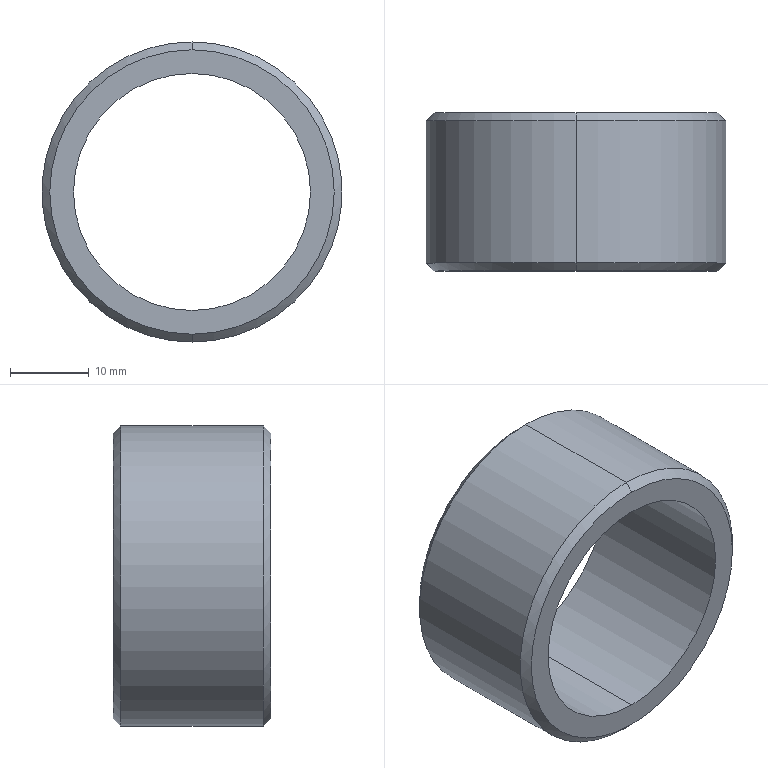Part | SolidWorks | features Chamfer 1, Extrusion 1 | 1 solid | 10 faces | box 38 x 20 x 38 mm | volume 8428 mm3 | cone 4 | cylinder 4 | plane 2 | commonest cylinder face diameters 30 x2 38 x2
STEP:
#1=CARTESIAN_POINT('',(0.,20.,18.));
#2=VERTEX_POINT('',#1);
#3=CARTESIAN_POINT('',(0.,20.,-18.));
#4=VERTEX_POINT('',#3);
#5=CARTESIAN_POINT('',(0.,20.,0.));
#6=DIRECTION('',(0.,1.,0.));
#7=DIRECTION('',(0.,0.,1.));
#8=AXIS2_PLACEMENT_3D('',#5,#6,#7);
#9=CIRCLE('',#8,18.);
#10=EDGE_CURVE('',#2,#4,#9,.T.);
#11=ORIENTED_EDGE('',*,*,#10,.F.);
#12=CARTESIAN_POINT('',(0.,19.,19.));
#13=VERTEX_POINT('',#12);
#14=CARTESIAN_POINT('',(0.,20.,18.));
#15=DIRECTION('',(0.,-0.7071,0.7071));
#16=VECTOR('',#15,1000.);
#17=LINE('',#14,#16);
#18=EDGE_CURVE('',#2,#13,#17,.T.);
#19=ORIENTED_EDGE('',*,*,#18,.T.);
#20=CARTESIAN_POINT('',(0.,19.,-19.));
#21=VERTEX_POINT('',#20);
#22=CARTESIAN_POINT('',(0.,19.,0.));
#23=DIRECTION('',(0.,-1.,0.));
#24=DIRECTION('',(0.,0.,1.));
#25=AXIS2_PLACEMENT_3D('',#22,#23,#24);
#26=CIRCLE('',#25,19.);
#27=EDGE_CURVE('',#21,#13,#26,.T.);
#28=ORIENTED_EDGE('',*,*,#27,.F.);
#29=CARTESIAN_POINT('',(0.,20.,-18.));
#30=DIRECTION('',(0.,-0.7071,-0.7071));
#31=VECTOR('',#30,1000.);
#32=LINE('',#29,#31);
#33=EDGE_CURVE('',#4,#21,#32,.T.);
#34=ORIENTED_EDGE('',*,*,#33,.F.);
#35=EDGE_LOOP('',(#11,#19,#28,#34));
#36=FACE_OUTER_BOUND('',#35,.T.);
#37=CARTESIAN_POINT('',(0.,20.,0.));
#38=DIRECTION('',(0.,-1.,0.));
#39=DIRECTION('',(0.,0.,-1.));
#40=AXIS2_PLACEMENT_3D('',#37,#38,#39);
#41=CONICAL_SURFACE('',#40,18.,0.7854);
#42=ADVANCED_FACE('',(#36),#41,.T.);
#43=CARTESIAN_POINT('',(0.,0.,-18.));
#44=VERTEX_POINT('',#43);
#45=CARTESIAN_POINT('',(0.,0.,18.));
#46=VERTEX_POINT('',#45);
#47=CARTESIAN_POINT('',(0.,0.,0.));
#48=DIRECTION('',(0.,-1.,0.));
#49=DIRECTION('',(0.,0.,1.));
#50=AXIS2_PLACEMENT_3D('',#47,#48,#49);
#51=CIRCLE('',#50,18.);
#52=EDGE_CURVE('',#44,#46,#51,.T.);
#53=ORIENTED_EDGE('',*,*,#52,.F.);
#54=CARTESIAN_POINT('',(0.,1.,-19.));
#55=VERTEX_POINT('',#54);
#56=CARTESIAN_POINT('',(0.,1.,-19.));
#57=DIRECTION('',(0.,0.7071,-0.7071));
#58=VECTOR('',#57,1000.);
#59=LINE('',#56,#58);
#60=EDGE_CURVE('',#44,#55,#59,.T.);
#61=ORIENTED_EDGE('',*,*,#60,.T.);
#62=CARTESIAN_POINT('',(0.,1.,19.));
#63=VERTEX_POINT('',#62);
#64=CARTESIAN_POINT('',(0.,1.,0.));
#65=DIRECTION('',(0.,1.,0.));
#66=DIRECTION('',(0.,0.,1.));
#67=AXIS2_PLACEMENT_3D('',#64,#65,#66);
#68=CIRCLE('',#67,19.);
#69=EDGE_CURVE('',#63,#55,#68,.T.);
#70=ORIENTED_EDGE('',*,*,#69,.F.);
#71=CARTESIAN_POINT('',(0.,1.,19.));
#72=DIRECTION('',(0.,0.7071,0.7071));
#73=VECTOR('',#72,1000.);
#74=LINE('',#71,#73);
#75=EDGE_CURVE('',#46,#63,#74,.T.);
#76=ORIENTED_EDGE('',*,*,#75,.F.);
#77=EDGE_LOOP('',(#53,#61,#70,#76));
#78=FACE_OUTER_BOUND('',#77,.T.);
#79=CARTESIAN_POINT('',(0.,1.,0.));
#80=DIRECTION('',(0.,1.,0.));
#81=DIRECTION('',(0.,0.,1.));
#82=AXIS2_PLACEMENT_3D('',#79,#80,#81);
#83=CONICAL_SURFACE('',#82,19.,0.7854);
#84=ADVANCED_FACE('',(#78),#83,.T.);
#85=CARTESIAN_POINT('',(0.,20.,-15.));
#86=VERTEX_POINT('',#85);
#87=CARTESIAN_POINT('',(0.,20.,15.));
#88=VERTEX_POINT('',#87);
#89=CARTESIAN_POINT('',(0.,20.,0.));
#90=DIRECTION('',(0.,1.,0.));
#91=DIRECTION('',(0.,0.,1.));
#92=AXIS2_PLACEMENT_3D('',#89,#90,#91);
#93=CIRCLE('',#92,15.);
#94=EDGE_CURVE('',#86,#88,#93,.T.);
#95=ORIENTED_EDGE('',*,*,#94,.T.);
#96=CARTESIAN_POINT('',(0.,0.,15.));
#97=VERTEX_POINT('',#96);
#98=CARTESIAN_POINT('',(0.,20.,15.));
#99=DIRECTION('',(0.,-1.,0.));
#100=VECTOR('',#99,1000.);
#101=LINE('',#98,#100);
#102=EDGE_CURVE('',#88,#97,#101,.T.);
#103=ORIENTED_EDGE('',*,*,#102,.T.);
#104=CARTESIAN_POINT('',(0.,0.,-15.));
#105=VERTEX_POINT('',#104);
#106=CARTESIAN_POINT('',(0.,0.,0.));
#107=DIRECTION('',(0.,1.,0.));
#108=DIRECTION('',(0.,0.,1.));
#109=AXIS2_PLACEMENT_3D('',#106,#107,#108);
#110=CIRCLE('',#109,15.);
#111=EDGE_CURVE('',#105,#97,#110,.T.);
#112=ORIENTED_EDGE('',*,*,#111,.F.);
#113=CARTESIAN_POINT('',(0.,20.,-15.));
#114=DIRECTION('',(0.,-1.,0.));
#115=VECTOR('',#114,1000.);
#116=LINE('',#113,#115);
#117=EDGE_CURVE('',#86,#105,#116,.T.);
#118=ORIENTED_EDGE('',*,*,#117,.F.);
#119=EDGE_LOOP('',(#95,#103,#112,#118));
#120=FACE_OUTER_BOUND('',#119,.T.);
#121=CARTESIAN_POINT('',(0.,20.,0.));
#122=DIRECTION('',(0.,-1.,0.));
#123=DIRECTION('',(0.,0.,-1.));
#124=AXIS2_PLACEMENT_3D('',#121,#122,#123);
#125=CYLINDRICAL_SURFACE('',#124,15.);
#126=ADVANCED_FACE('',(#120),#125,.F.);
#127=ORIENTED_EDGE('',*,*,#27,.T.);
#128=CARTESIAN_POINT('',(0.,20.,19.));
#129=DIRECTION('',(0.,-1.,0.));
#130=VECTOR('',#129,1000.);
#131=LINE('',#128,#130);
#132=EDGE_CURVE('',#13,#63,#131,.T.);
#133=ORIENTED_EDGE('',*,*,#132,.T.);
#134=ORIENTED_EDGE('',*,*,#69,.T.);
#135=CARTESIAN_POINT('',(0.,20.,-19.));
#136=DIRECTION('',(0.,-1.,0.));
#137=VECTOR('',#136,1000.);
#138=LINE('',#135,#137);
#139=EDGE_CURVE('',#21,#55,#138,.T.);
#140=ORIENTED_EDGE('',*,*,#139,.F.);
#141=EDGE_LOOP('',(#127,#133,#134,#140));
#142=FACE_OUTER_BOUND('',#141,.T.);
#143=CARTESIAN_POINT('',(0.,20.,0.));
#144=DIRECTION('',(0.,-1.,0.));
#145=DIRECTION('',(0.,0.,-1.));
#146=AXIS2_PLACEMENT_3D('',#143,#144,#145);
#147=CYLINDRICAL_SURFACE('',#146,19.);
#148=ADVANCED_FACE('',(#142),#147,.T.);
#149=CARTESIAN_POINT('',(0.,20.,0.));
#150=DIRECTION('',(0.,1.,0.));
#151=DIRECTION('',(0.,0.,1.));
#152=AXIS2_PLACEMENT_3D('',#149,#150,#151);
#153=CIRCLE('',#152,18.);
#154=EDGE_CURVE('',#4,#2,#153,.T.);
#155=ORIENTED_EDGE('',*,*,#154,.T.);
#156=ORIENTED_EDGE('',*,*,#10,.T.);
#157=EDGE_LOOP('',(#155,#156));
#158=FACE_OUTER_BOUND('',#157,.T.);
#159=ORIENTED_EDGE('',*,*,#94,.F.);
#160=CARTESIAN_POINT('',(0.,20.,0.));
#161=DIRECTION('',(0.,1.,0.));
#162=DIRECTION('',(0.,0.,1.));
#163=AXIS2_PLACEMENT_3D('',#160,#161,#162);
#164=CIRCLE('',#163,15.);
#165=EDGE_CURVE('',#88,#86,#164,.T.);
#166=ORIENTED_EDGE('',*,*,#165,.F.);
#167=EDGE_LOOP('',(#159,#166));
#168=FACE_BOUND('',#167,.T.);
#169=CARTESIAN_POINT('',(0.,20.,0.));
#170=DIRECTION('',(0.,1.,0.));
#171=DIRECTION('',(0.,0.,1.));
#172=AXIS2_PLACEMENT_3D('',#169,#170,#171);
#173=PLANE('',#172);
#174=ADVANCED_FACE('',(#158,#168),#173,.T.);
#175=CARTESIAN_POINT('',(0.,0.,0.));
#176=DIRECTION('',(0.,-1.,0.));
#177=DIRECTION('',(0.,0.,1.));
#178=AXIS2_PLACEMENT_3D('',#175,#176,#177);
#179=CIRCLE('',#178,18.);
#180=EDGE_CURVE('',#46,#44,#179,.T.);
#181=ORIENTED_EDGE('',*,*,#180,.T.);
#182=ORIENTED_EDGE('',*,*,#52,.T.);
#183=EDGE_LOOP('',(#181,#182));
#184=FACE_OUTER_BOUND('',#183,.T.);
#185=ORIENTED_EDGE('',*,*,#111,.T.);
#186=CARTESIAN_POINT('',(0.,0.,0.));
#187=DIRECTION('',(0.,1.,0.));
#188=DIRECTION('',(0.,0.,1.));
#189=AXIS2_PLACEMENT_3D('',#186,#187,#188);
#190=CIRCLE('',#189,15.);
#191=EDGE_CURVE('',#97,#105,#190,.T.);
#192=ORIENTED_EDGE('',*,*,#191,.T.);
#193=EDGE_LOOP('',(#185,#192));
#194=FACE_BOUND('',#193,.T.);
#195=CARTESIAN_POINT('',(0.,0.,0.));
#196=DIRECTION('',(0.,1.,0.));
#197=DIRECTION('',(0.,0.,1.));
#198=AXIS2_PLACEMENT_3D('',#195,#196,#197);
#199=PLANE('',#198);
#200=ADVANCED_FACE('',(#184,#194),#199,.F.);
#201=ORIENTED_EDGE('',*,*,#132,.F.);
#202=CARTESIAN_POINT('',(0.,19.,0.));
#203=DIRECTION('',(0.,-1.,0.));
#204=DIRECTION('',(0.,0.,1.));
#205=AXIS2_PLACEMENT_3D('',#202,#203,#204);
#206=CIRCLE('',#205,19.);
#207=EDGE_CURVE('',#13,#21,#206,.T.);
#208=ORIENTED_EDGE('',*,*,#207,.T.);
#209=ORIENTED_EDGE('',*,*,#139,.T.);
#210=CARTESIAN_POINT('',(0.,1.,0.));
#211=DIRECTION('',(0.,1.,0.));
#212=DIRECTION('',(0.,0.,1.));
#213=AXIS2_PLACEMENT_3D('',#210,#211,#212);
#214=CIRCLE('',#213,19.);
#215=EDGE_CURVE('',#55,#63,#214,.T.);
#216=ORIENTED_EDGE('',*,*,#215,.T.);
#217=EDGE_LOOP('',(#201,#208,#209,#216));
#218=FACE_OUTER_BOUND('',#217,.T.);
#219=CARTESIAN_POINT('',(0.,20.,0.));
#220=DIRECTION('',(0.,-1.,0.));
#221=DIRECTION('',(0.,0.,-1.));
#222=AXIS2_PLACEMENT_3D('',#219,#220,#221);
#223=CYLINDRICAL_SURFACE('',#222,19.);
#224=ADVANCED_FACE('',(#218),#223,.T.);
#225=ORIENTED_EDGE('',*,*,#102,.F.);
#226=ORIENTED_EDGE('',*,*,#165,.T.);
#227=ORIENTED_EDGE('',*,*,#117,.T.);
#228=ORIENTED_EDGE('',*,*,#191,.F.);
#229=EDGE_LOOP('',(#225,#226,#227,#228));
#230=FACE_OUTER_BOUND('',#229,.T.);
#231=CARTESIAN_POINT('',(0.,20.,0.));
#232=DIRECTION('',(0.,-1.,0.));
#233=DIRECTION('',(0.,0.,-1.));
#234=AXIS2_PLACEMENT_3D('',#231,#232,#233);
#235=CYLINDRICAL_SURFACE('',#234,15.);
#236=ADVANCED_FACE('',(#230),#235,.F.);
#237=ORIENTED_EDGE('',*,*,#60,.F.);
#238=ORIENTED_EDGE('',*,*,#180,.F.);
#239=ORIENTED_EDGE('',*,*,#75,.T.);
#240=ORIENTED_EDGE('',*,*,#215,.F.);
#241=EDGE_LOOP('',(#237,#238,#239,#240));
#242=FACE_OUTER_BOUND('',#241,.T.);
#243=CARTESIAN_POINT('',(0.,1.,0.));
#244=DIRECTION('',(0.,1.,0.));
#245=DIRECTION('',(0.,0.,1.));
#246=AXIS2_PLACEMENT_3D('',#243,#244,#245);
#247=CONICAL_SURFACE('',#246,19.,0.7854);
#248=ADVANCED_FACE('',(#242),#247,.T.);
#249=ORIENTED_EDGE('',*,*,#18,.F.);
#250=ORIENTED_EDGE('',*,*,#154,.F.);
#251=ORIENTED_EDGE('',*,*,#33,.T.);
#252=ORIENTED_EDGE('',*,*,#207,.F.);
#253=EDGE_LOOP('',(#249,#250,#251,#252));
#254=FACE_OUTER_BOUND('',#253,.T.);
#255=CARTESIAN_POINT('',(0.,20.,0.));
#256=DIRECTION('',(0.,-1.,0.));
#257=DIRECTION('',(0.,0.,-1.));
#258=AXIS2_PLACEMENT_3D('',#255,#256,#257);
#259=CONICAL_SURFACE('',#258,18.,0.7854);
#260=ADVANCED_FACE('',(#254),#259,.T.);
#261=CLOSED_SHELL('',(#42,#84,#126,#148,#174,#200,#224,#236,#248,#260));
#262=MANIFOLD_SOLID_BREP('',#261);
#263=CARTESIAN_POINT('',(0.,0.,0.));
#264=DIRECTION('',(0.,0.,1.));
#265=DIRECTION('',(1.,0.,0.));
#266=AXIS2_PLACEMENT_3D('',#263,#264,#265);
#267=(LENGTH_UNIT()NAMED_UNIT(*)SI_UNIT(.MILLI.,.METRE.));
#268=UNCERTAINTY_MEASURE_WITH_UNIT(LENGTH_MEASURE(0.00001),#267,'','');
#269=(NAMED_UNIT(*)PLANE_ANGLE_UNIT()SI_UNIT($,.RADIAN.));
#270=(NAMED_UNIT(*)SI_UNIT($,.STERADIAN.)SOLID_ANGLE_UNIT());
#271=(GEOMETRIC_REPRESENTATION_CONTEXT(3)GLOBAL_UNCERTAINTY_ASSIGNED_CONTEXT((#268))GLOBAL_UNIT_ASSIGNED_CONTEXT((#267,#269,#270))REPRESENTATION_CONTEXT('',''));
#272=ADVANCED_BREP_SHAPE_REPRESENTATION('',(#262,#266),#271);